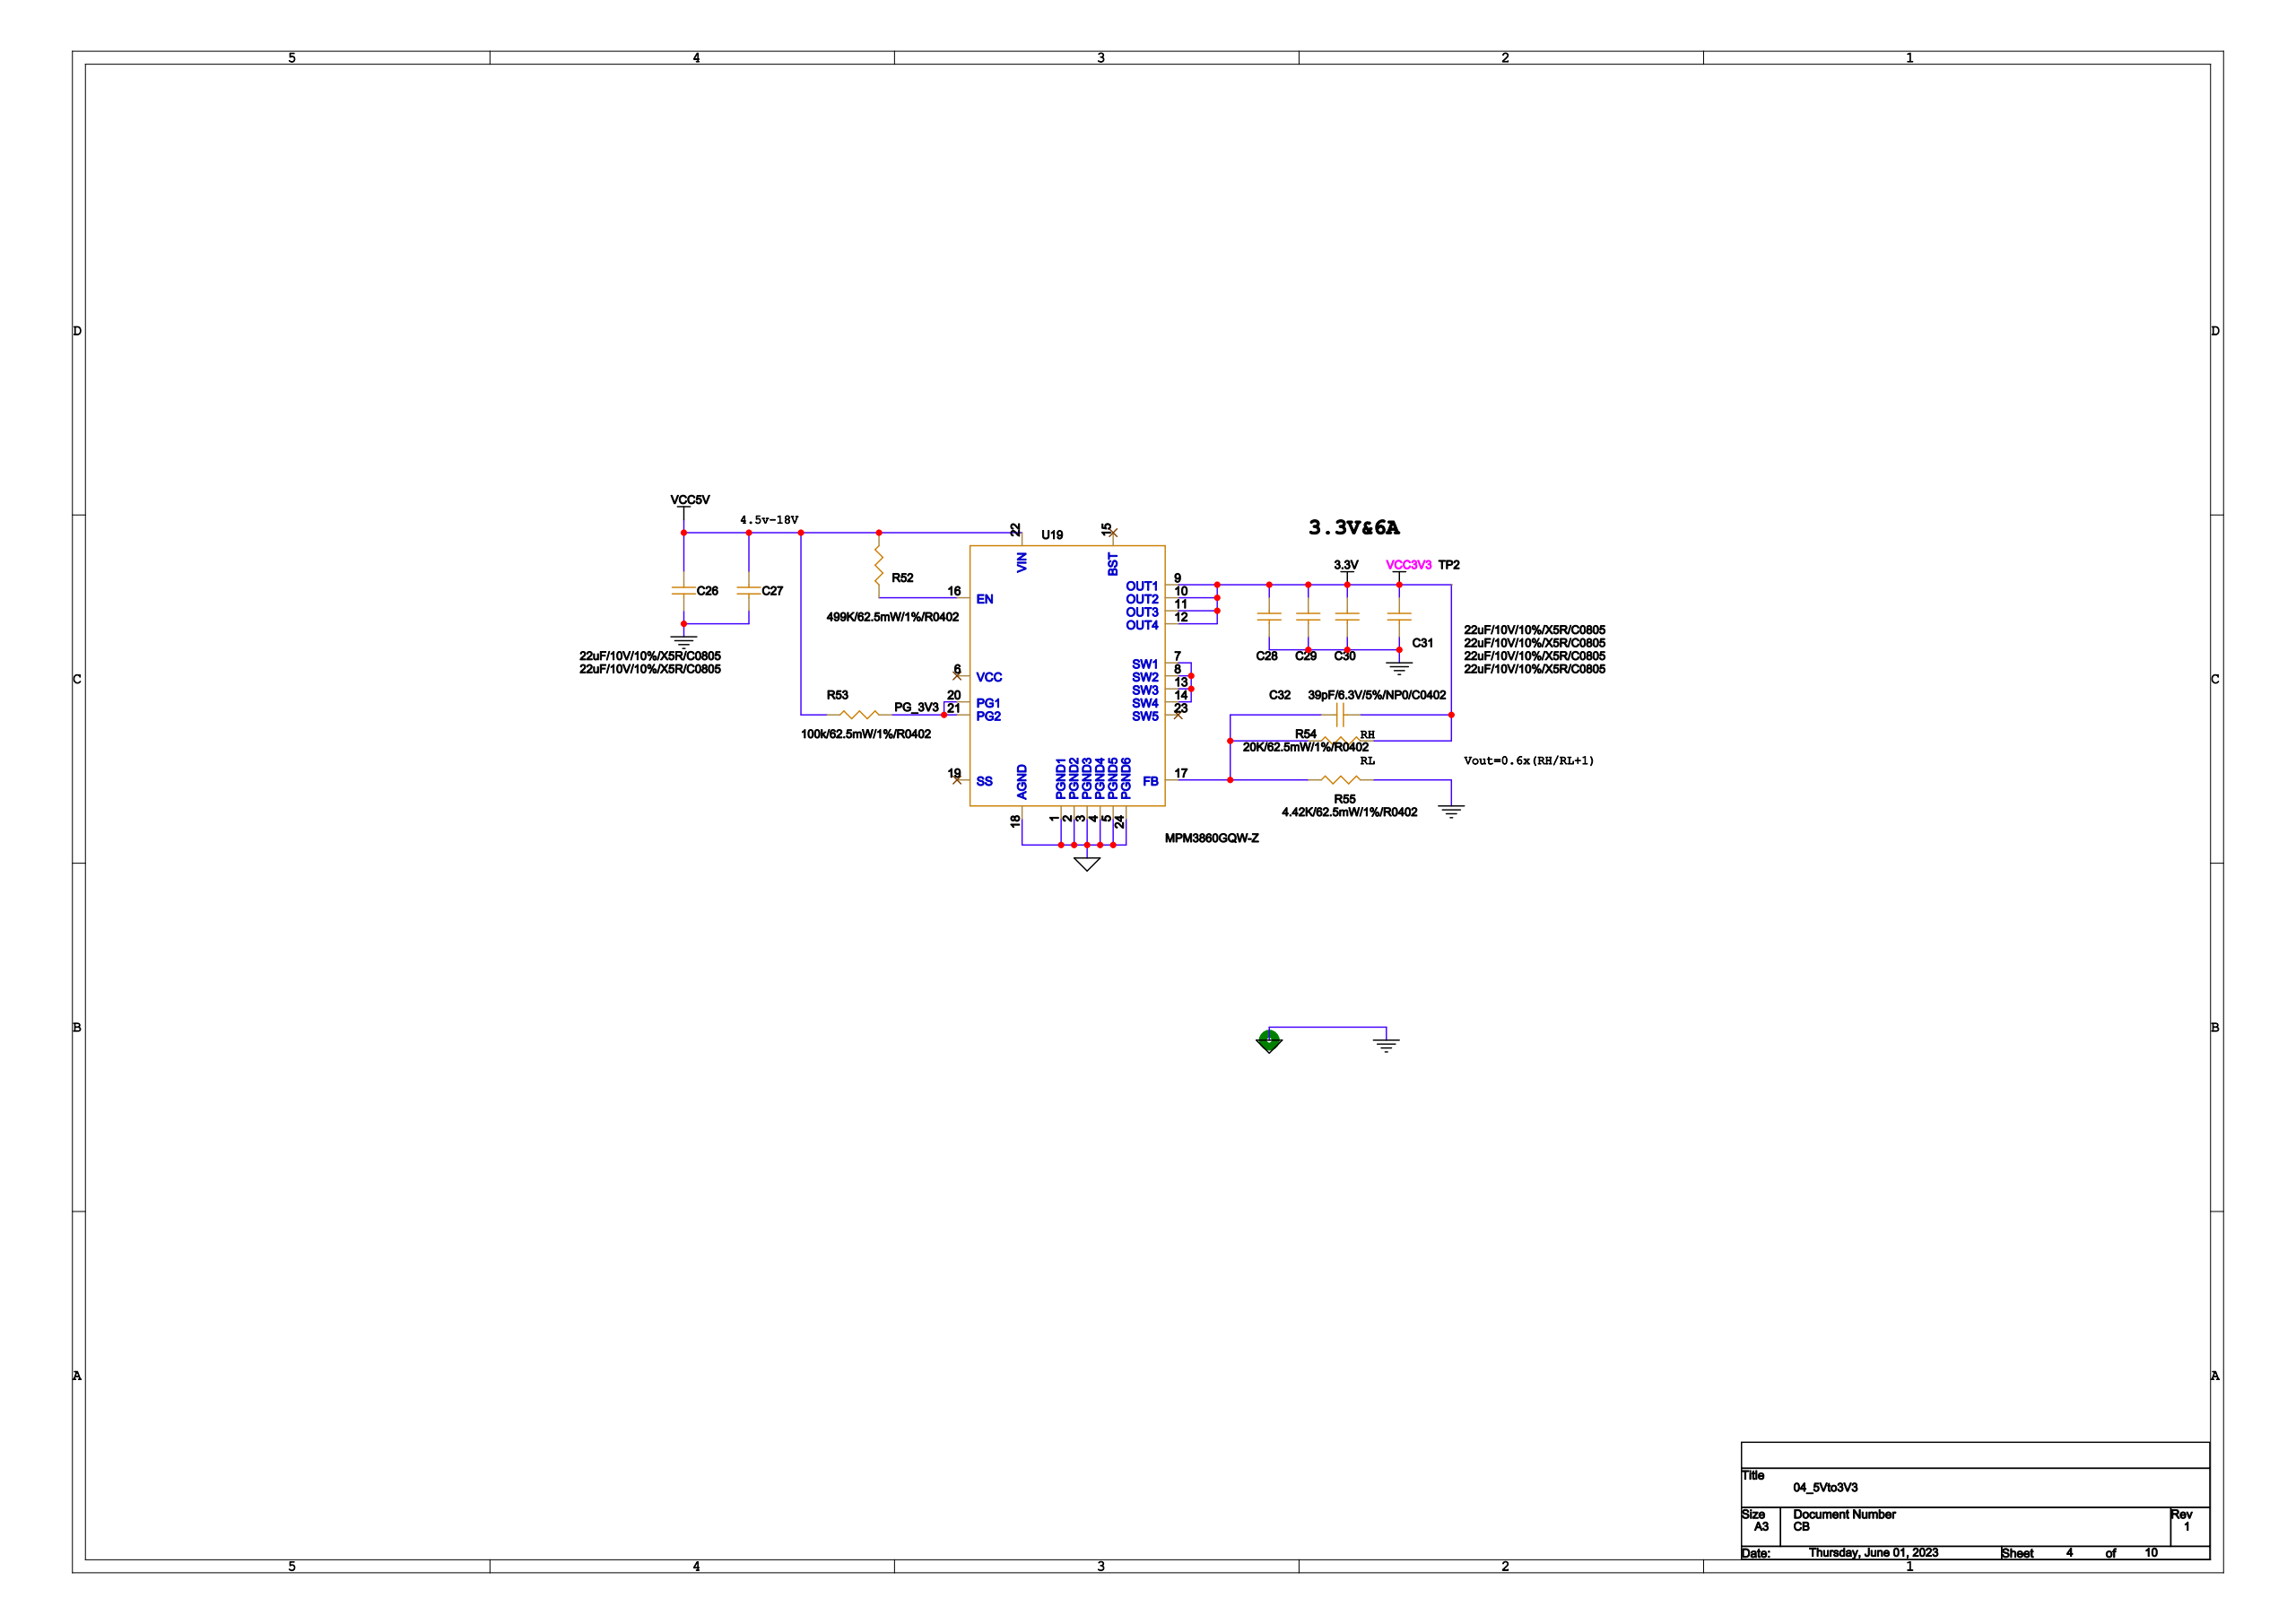Circuit board | Cadence Allegro | 480 parts | 625 nets | one sheet of the schematic
Parts on this sheet (reference | value | footprint):
C26 | 22uF/10V/10%/X5R/C0805 | 0805
C27 | 22uF/10V/10%/X5R/C0805 | 0805
C28 | 22uF/10V/10%/X5R/C0805 | 0805
C29 | 22uF/10V/10%/X5R/C0805 | 0805
C30 | 22uF/10V/10%/X5R/C0805 | 0805
C31 | 22uF/10V/10%/X5R/C0805 | 0805
C32 | 39pF/6.3V/5%/NP0/C0402 | 0402
R52 | 499K/62.5mW/1%/R0402 | 0402
R53 | 100k/62.5mW/1%/R0402 | 0402
R54 | 20K/62.5mW/1%/R0402 | 0402
R55 | 4.42K/62.5mW/1%/R0402 | 0402
SW1 | SW DIP-6 | W-SMD_12P-L9_3-W5_4-P1_27-LS2
TP2 | TEST POINT A | TEST_12MM
U19 | MPM3860GQW-Z | MPM3650GQW
Nets of these parts (net: part-pin ...):
AGND: C26-2 C27-2 C28-2 C29-2 C30-2 C31-2 R55-1 SW1-7 SW1-8 SW1-9 SW1-10 SW1-11 SW1-12 U19-1 U19-2 U19-3 U19-4 U19-5 U19-18 U19-24
3.3V: C28-1 C29-1 C30-1 C31-1 C32-2 R54-1 TP2-1 U19-9 U19-10 U19-11 U19-12
BANK33_L17_P: SW1-1
BANK33_L17_N: SW1-2
BANK33_L18_P: SW1-3
BANK33_L18_N: SW1-4
BANK33_L24_N: SW1-5
BANK33_L24_P: SW1-6
VCC5V: C26-1 C27-1 R52-1 R53-2 U19-22
N23155169: C32-1 R54-2 R55-2 U19-17
N23155064: R52-2 U19-16
PG_3V3: R53-1 U19-20 U19-21
N23155134: U19-7 U19-8 U19-13 U19-14